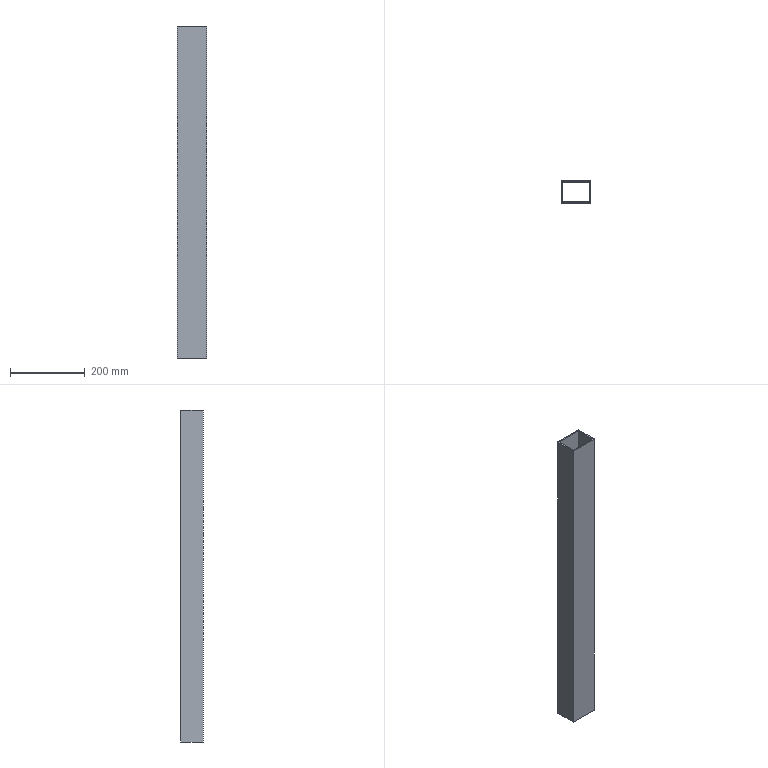Part | STEP file | Guide wheel mechanism revised.sldasm-Part-30 | 1 solid | 12 faces | box 80 x 60 x 890 mm | volume 705411 mm3 | plane 11 | cylinder 1 | commonest cylinder face diameters 500 x1
STEP:
#1=CARTESIAN_POINT('',(-485.,760.,445.));
#2=VERTEX_POINT('',#1);
#3=CARTESIAN_POINT('',(-405.,760.,445.));
#4=VERTEX_POINT('',#3);
#5=CARTESIAN_POINT('',(-405.,760.,445.));
#6=DIRECTION('',(1.,0.,0.));
#7=VECTOR('',#6,1000.);
#8=LINE('',#5,#7);
#9=EDGE_CURVE('',#2,#4,#8,.T.);
#10=ORIENTED_EDGE('',*,*,#9,.F.);
#11=CARTESIAN_POINT('',(-485.,760.,-445.));
#12=VERTEX_POINT('',#11);
#13=CARTESIAN_POINT('',(-485.,760.,545.));
#14=DIRECTION('',(0.,0.,-1.));
#15=VECTOR('',#14,1000.);
#16=LINE('',#13,#15);
#17=EDGE_CURVE('',#2,#12,#16,.T.);
#18=ORIENTED_EDGE('',*,*,#17,.T.);
#19=CARTESIAN_POINT('',(-405.,760.,-445.));
#20=VERTEX_POINT('',#19);
#21=CARTESIAN_POINT('',(-405.,760.,-445.));
#22=DIRECTION('',(1.,0.,0.));
#23=VECTOR('',#22,1000.);
#24=LINE('',#21,#23);
#25=EDGE_CURVE('',#12,#20,#24,.T.);
#26=ORIENTED_EDGE('',*,*,#25,.T.);
#27=CARTESIAN_POINT('',(-405.,760.,545.));
#28=DIRECTION('',(0.,0.,-1.));
#29=VECTOR('',#28,1000.);
#30=LINE('',#27,#29);
#31=EDGE_CURVE('',#4,#20,#30,.T.);
#32=ORIENTED_EDGE('',*,*,#31,.F.);
#33=EDGE_LOOP('',(#10,#18,#26,#32));
#34=FACE_OUTER_BOUND('',#33,.T.);
#35=CARTESIAN_POINT('',(-405.,760.,545.));
#36=DIRECTION('',(0.,1.,0.));
#37=DIRECTION('',(0.,0.,1.));
#38=AXIS2_PLACEMENT_3D('',#35,#36,#37);
#39=PLANE('',#38);
#40=ADVANCED_FACE('',(#34),#39,.F.);
#41=CARTESIAN_POINT('',(-485.,820.,445.));
#42=VERTEX_POINT('',#41);
#43=CARTESIAN_POINT('',(-485.,820.,445.));
#44=DIRECTION('',(0.,-1.,0.));
#45=VECTOR('',#44,1000.);
#46=LINE('',#43,#45);
#47=EDGE_CURVE('',#42,#2,#46,.T.);
#48=ORIENTED_EDGE('',*,*,#47,.F.);
#49=CARTESIAN_POINT('',(-485.,820.,-445.));
#50=VERTEX_POINT('',#49);
#51=CARTESIAN_POINT('',(-485.,820.,545.));
#52=DIRECTION('',(0.,0.,-1.));
#53=VECTOR('',#52,1000.);
#54=LINE('',#51,#53);
#55=EDGE_CURVE('',#42,#50,#54,.T.);
#56=ORIENTED_EDGE('',*,*,#55,.T.);
#57=CARTESIAN_POINT('',(-485.,820.,-445.));
#58=DIRECTION('',(0.,-1.,0.));
#59=VECTOR('',#58,1000.);
#60=LINE('',#57,#59);
#61=EDGE_CURVE('',#50,#12,#60,.T.);
#62=ORIENTED_EDGE('',*,*,#61,.T.);
#63=ORIENTED_EDGE('',*,*,#17,.F.);
#64=EDGE_LOOP('',(#48,#56,#62,#63));
#65=FACE_OUTER_BOUND('',#64,.T.);
#66=CARTESIAN_POINT('',(-485.,820.,545.));
#67=DIRECTION('',(1.,0.,0.));
#68=DIRECTION('',(0.,0.,-1.));
#69=AXIS2_PLACEMENT_3D('',#66,#67,#68);
#70=PLANE('',#69);
#71=ADVANCED_FACE('',(#65),#70,.F.);
#72=CARTESIAN_POINT('',(-405.,820.,445.));
#73=VERTEX_POINT('',#72);
#74=CARTESIAN_POINT('',(-405.,820.,267.168));
#75=VERTEX_POINT('',#74);
#76=CARTESIAN_POINT('',(-405.,820.,545.));
#77=DIRECTION('',(0.,0.,-1.));
#78=VECTOR('',#77,1000.);
#79=LINE('',#76,#78);
#80=EDGE_CURVE('',#73,#75,#79,.T.);
#81=ORIENTED_EDGE('',*,*,#80,.T.);
#82=CARTESIAN_POINT('',(-405.,820.,25.252));
#83=VERTEX_POINT('',#82);
#84=CARTESIAN_POINT('',(-186.21,820.,146.21));
#85=DIRECTION('',(0.,-1.,0.));
#86=DIRECTION('',(0.,0.,-1.));
#87=AXIS2_PLACEMENT_3D('',#84,#85,#86);
#88=CIRCLE('',#87,250.);
#89=EDGE_CURVE('',#75,#83,#88,.T.);
#90=ORIENTED_EDGE('',*,*,#89,.T.);
#91=CARTESIAN_POINT('',(-405.,820.,-445.));
#92=VERTEX_POINT('',#91);
#93=CARTESIAN_POINT('',(-405.,820.,545.));
#94=DIRECTION('',(0.,0.,-1.));
#95=VECTOR('',#94,1000.);
#96=LINE('',#93,#95);
#97=EDGE_CURVE('',#83,#92,#96,.T.);
#98=ORIENTED_EDGE('',*,*,#97,.T.);
#99=CARTESIAN_POINT('',(-405.,820.,-445.));
#100=DIRECTION('',(-1.,0.,0.));
#101=VECTOR('',#100,1000.);
#102=LINE('',#99,#101);
#103=EDGE_CURVE('',#92,#50,#102,.T.);
#104=ORIENTED_EDGE('',*,*,#103,.T.);
#105=ORIENTED_EDGE('',*,*,#55,.F.);
#106=CARTESIAN_POINT('',(-405.,820.,445.));
#107=DIRECTION('',(-1.,0.,0.));
#108=VECTOR('',#107,1000.);
#109=LINE('',#106,#108);
#110=EDGE_CURVE('',#73,#42,#109,.T.);
#111=ORIENTED_EDGE('',*,*,#110,.F.);
#112=EDGE_LOOP('',(#81,#90,#98,#104,#105,#111));
#113=FACE_OUTER_BOUND('',#112,.T.);
#114=CARTESIAN_POINT('',(-405.,820.,545.));
#115=DIRECTION('',(0.,-1.,0.));
#116=DIRECTION('',(0.,0.,-1.));
#117=AXIS2_PLACEMENT_3D('',#114,#115,#116);
#118=PLANE('',#117);
#119=ADVANCED_FACE('',(#113),#118,.F.);
#120=CARTESIAN_POINT('',(-405.,818.01,267.168));
#121=VERTEX_POINT('',#120);
#122=CARTESIAN_POINT('',(-405.,818.01,25.252));
#123=VERTEX_POINT('',#122);
#124=CARTESIAN_POINT('',(-405.,818.01,545.));
#125=DIRECTION('',(0.,0.,-1.));
#126=VECTOR('',#125,1000.);
#127=LINE('',#124,#126);
#128=EDGE_CURVE('',#121,#123,#127,.T.);
#129=ORIENTED_EDGE('',*,*,#128,.F.);
#130=CARTESIAN_POINT('',(-405.,818.01,267.168));
#131=DIRECTION('',(0.,1.,0.));
#132=VECTOR('',#131,1000.);
#133=LINE('',#130,#132);
#134=EDGE_CURVE('',#121,#75,#133,.T.);
#135=ORIENTED_EDGE('',*,*,#134,.T.);
#136=ORIENTED_EDGE('',*,*,#80,.F.);
#137=CARTESIAN_POINT('',(-405.,820.,445.));
#138=DIRECTION('',(0.,1.,0.));
#139=VECTOR('',#138,1000.);
#140=LINE('',#137,#139);
#141=EDGE_CURVE('',#4,#73,#140,.T.);
#142=ORIENTED_EDGE('',*,*,#141,.F.);
#143=ORIENTED_EDGE('',*,*,#31,.T.);
#144=CARTESIAN_POINT('',(-405.,820.,-445.));
#145=DIRECTION('',(0.,1.,0.));
#146=VECTOR('',#145,1000.);
#147=LINE('',#144,#146);
#148=EDGE_CURVE('',#20,#92,#147,.T.);
#149=ORIENTED_EDGE('',*,*,#148,.T.);
#150=ORIENTED_EDGE('',*,*,#97,.F.);
#151=CARTESIAN_POINT('',(-405.,818.01,25.252));
#152=DIRECTION('',(0.,-1.,0.));
#153=VECTOR('',#152,1000.);
#154=LINE('',#151,#153);
#155=EDGE_CURVE('',#83,#123,#154,.T.);
#156=ORIENTED_EDGE('',*,*,#155,.T.);
#157=EDGE_LOOP('',(#129,#135,#136,#142,#143,#149,#150,#156));
#158=FACE_OUTER_BOUND('',#157,.T.);
#159=CARTESIAN_POINT('',(-405.,820.,545.));
#160=DIRECTION('',(-1.,0.,0.));
#161=DIRECTION('',(0.,0.,1.));
#162=AXIS2_PLACEMENT_3D('',#159,#160,#161);
#163=PLANE('',#162);
#164=ADVANCED_FACE('',(#158),#163,.F.);
#165=ORIENTED_EDGE('',*,*,#148,.F.);
#166=ORIENTED_EDGE('',*,*,#25,.F.);
#167=ORIENTED_EDGE('',*,*,#61,.F.);
#168=ORIENTED_EDGE('',*,*,#103,.F.);
#169=EDGE_LOOP('',(#165,#166,#167,#168));
#170=FACE_OUTER_BOUND('',#169,.T.);
#171=CARTESIAN_POINT('',(-482.,763.,-445.));
#172=VERTEX_POINT('',#171);
#173=CARTESIAN_POINT('',(-408.,763.,-445.));
#174=VERTEX_POINT('',#173);
#175=CARTESIAN_POINT('',(-408.,763.,-445.));
#176=DIRECTION('',(1.,0.,0.));
#177=VECTOR('',#176,1000.);
#178=LINE('',#175,#177);
#179=EDGE_CURVE('',#172,#174,#178,.T.);
#180=ORIENTED_EDGE('',*,*,#179,.T.);
#181=CARTESIAN_POINT('',(-408.,817.,-445.));
#182=VERTEX_POINT('',#181);
#183=CARTESIAN_POINT('',(-408.,817.,-445.));
#184=DIRECTION('',(0.,1.,0.));
#185=VECTOR('',#184,1000.);
#186=LINE('',#183,#185);
#187=EDGE_CURVE('',#174,#182,#186,.T.);
#188=ORIENTED_EDGE('',*,*,#187,.T.);
#189=CARTESIAN_POINT('',(-482.,817.,-445.));
#190=VERTEX_POINT('',#189);
#191=CARTESIAN_POINT('',(-408.,817.,-445.));
#192=DIRECTION('',(-1.,0.,0.));
#193=VECTOR('',#192,1000.);
#194=LINE('',#191,#193);
#195=EDGE_CURVE('',#182,#190,#194,.T.);
#196=ORIENTED_EDGE('',*,*,#195,.T.);
#197=CARTESIAN_POINT('',(-482.,817.,-445.));
#198=DIRECTION('',(0.,-1.,0.));
#199=VECTOR('',#198,1000.);
#200=LINE('',#197,#199);
#201=EDGE_CURVE('',#190,#172,#200,.T.);
#202=ORIENTED_EDGE('',*,*,#201,.T.);
#203=EDGE_LOOP('',(#180,#188,#196,#202));
#204=FACE_BOUND('',#203,.T.);
#205=CARTESIAN_POINT('',(0.,0.,-445.));
#206=DIRECTION('',(0.,0.,-1.));
#207=DIRECTION('',(-1.,0.,0.));
#208=AXIS2_PLACEMENT_3D('',#205,#206,#207);
#209=PLANE('',#208);
#210=ADVANCED_FACE('',(#170,#204),#209,.T.);
#211=CARTESIAN_POINT('',(-482.,763.,445.));
#212=VERTEX_POINT('',#211);
#213=CARTESIAN_POINT('',(-482.,763.,545.));
#214=DIRECTION('',(0.,0.,-1.));
#215=VECTOR('',#214,1000.);
#216=LINE('',#213,#215);
#217=EDGE_CURVE('',#212,#172,#216,.T.);
#218=ORIENTED_EDGE('',*,*,#217,.F.);
#219=CARTESIAN_POINT('',(-408.,763.,445.));
#220=VERTEX_POINT('',#219);
#221=CARTESIAN_POINT('',(-408.,763.,445.));
#222=DIRECTION('',(1.,0.,0.));
#223=VECTOR('',#222,1000.);
#224=LINE('',#221,#223);
#225=EDGE_CURVE('',#212,#220,#224,.T.);
#226=ORIENTED_EDGE('',*,*,#225,.T.);
#227=CARTESIAN_POINT('',(-408.,763.,545.));
#228=DIRECTION('',(0.,0.,-1.));
#229=VECTOR('',#228,1000.);
#230=LINE('',#227,#229);
#231=EDGE_CURVE('',#220,#174,#230,.T.);
#232=ORIENTED_EDGE('',*,*,#231,.T.);
#233=ORIENTED_EDGE('',*,*,#179,.F.);
#234=EDGE_LOOP('',(#218,#226,#232,#233));
#235=FACE_OUTER_BOUND('',#234,.T.);
#236=CARTESIAN_POINT('',(-408.,763.,545.));
#237=DIRECTION('',(0.,1.,0.));
#238=DIRECTION('',(0.,0.,1.));
#239=AXIS2_PLACEMENT_3D('',#236,#237,#238);
#240=PLANE('',#239);
#241=ADVANCED_FACE('',(#235),#240,.T.);
#242=CARTESIAN_POINT('',(-482.,817.,445.));
#243=VERTEX_POINT('',#242);
#244=CARTESIAN_POINT('',(-482.,817.,545.));
#245=DIRECTION('',(0.,0.,-1.));
#246=VECTOR('',#245,1000.);
#247=LINE('',#244,#246);
#248=EDGE_CURVE('',#243,#190,#247,.T.);
#249=ORIENTED_EDGE('',*,*,#248,.F.);
#250=CARTESIAN_POINT('',(-482.,817.,445.));
#251=DIRECTION('',(0.,-1.,0.));
#252=VECTOR('',#251,1000.);
#253=LINE('',#250,#252);
#254=EDGE_CURVE('',#243,#212,#253,.T.);
#255=ORIENTED_EDGE('',*,*,#254,.T.);
#256=ORIENTED_EDGE('',*,*,#217,.T.);
#257=ORIENTED_EDGE('',*,*,#201,.F.);
#258=EDGE_LOOP('',(#249,#255,#256,#257));
#259=FACE_OUTER_BOUND('',#258,.T.);
#260=CARTESIAN_POINT('',(-482.,817.,545.));
#261=DIRECTION('',(1.,0.,0.));
#262=DIRECTION('',(0.,0.,-1.));
#263=AXIS2_PLACEMENT_3D('',#260,#261,#262);
#264=PLANE('',#263);
#265=ADVANCED_FACE('',(#259),#264,.T.);
#266=CARTESIAN_POINT('',(-408.,817.,445.));
#267=VERTEX_POINT('',#266);
#268=CARTESIAN_POINT('',(-408.,817.,545.));
#269=DIRECTION('',(0.,0.,-1.));
#270=VECTOR('',#269,1000.);
#271=LINE('',#268,#270);
#272=EDGE_CURVE('',#267,#182,#271,.T.);
#273=ORIENTED_EDGE('',*,*,#272,.F.);
#274=CARTESIAN_POINT('',(-408.,817.,445.));
#275=DIRECTION('',(-1.,0.,0.));
#276=VECTOR('',#275,1000.);
#277=LINE('',#274,#276);
#278=EDGE_CURVE('',#267,#243,#277,.T.);
#279=ORIENTED_EDGE('',*,*,#278,.T.);
#280=ORIENTED_EDGE('',*,*,#248,.T.);
#281=ORIENTED_EDGE('',*,*,#195,.F.);
#282=EDGE_LOOP('',(#273,#279,#280,#281));
#283=FACE_OUTER_BOUND('',#282,.T.);
#284=CARTESIAN_POINT('',(-408.,817.,545.));
#285=DIRECTION('',(0.,-1.,0.));
#286=DIRECTION('',(0.,0.,-1.));
#287=AXIS2_PLACEMENT_3D('',#284,#285,#286);
#288=PLANE('',#287);
#289=ADVANCED_FACE('',(#283),#288,.T.);
#290=ORIENTED_EDGE('',*,*,#231,.F.);
#291=CARTESIAN_POINT('',(-408.,817.,445.));
#292=DIRECTION('',(0.,1.,0.));
#293=VECTOR('',#292,1000.);
#294=LINE('',#291,#293);
#295=EDGE_CURVE('',#220,#267,#294,.T.);
#296=ORIENTED_EDGE('',*,*,#295,.T.);
#297=ORIENTED_EDGE('',*,*,#272,.T.);
#298=ORIENTED_EDGE('',*,*,#187,.F.);
#299=EDGE_LOOP('',(#290,#296,#297,#298));
#300=FACE_OUTER_BOUND('',#299,.T.);
#301=CARTESIAN_POINT('',(-408.,817.,545.));
#302=DIRECTION('',(-1.,0.,0.));
#303=DIRECTION('',(0.,-1.,0.));
#304=AXIS2_PLACEMENT_3D('',#301,#302,#303);
#305=PLANE('',#304);
#306=ADVANCED_FACE('',(#300),#305,.T.);
#307=ORIENTED_EDGE('',*,*,#295,.F.);
#308=ORIENTED_EDGE('',*,*,#225,.F.);
#309=ORIENTED_EDGE('',*,*,#254,.F.);
#310=ORIENTED_EDGE('',*,*,#278,.F.);
#311=EDGE_LOOP('',(#307,#308,#309,#310));
#312=FACE_BOUND('',#311,.T.);
#313=ORIENTED_EDGE('',*,*,#9,.T.);
#314=ORIENTED_EDGE('',*,*,#141,.T.);
#315=ORIENTED_EDGE('',*,*,#110,.T.);
#316=ORIENTED_EDGE('',*,*,#47,.T.);
#317=EDGE_LOOP('',(#313,#314,#315,#316));
#318=FACE_OUTER_BOUND('',#317,.T.);
#319=CARTESIAN_POINT('',(-405.,1970.,445.));
#320=DIRECTION('',(0.,0.,1.));
#321=DIRECTION('',(1.,0.,0.));
#322=AXIS2_PLACEMENT_3D('',#319,#320,#321);
#323=PLANE('',#322);
#324=ADVANCED_FACE('',(#312,#318),#323,.T.);
#325=CARTESIAN_POINT('',(-186.21,818.01,146.21));
#326=DIRECTION('',(0.,1.,0.));
#327=DIRECTION('',(0.,0.,1.));
#328=AXIS2_PLACEMENT_3D('',#325,#326,#327);
#329=CIRCLE('',#328,250.);
#330=EDGE_CURVE('',#123,#121,#329,.T.);
#331=ORIENTED_EDGE('',*,*,#330,.F.);
#332=ORIENTED_EDGE('',*,*,#155,.F.);
#333=ORIENTED_EDGE('',*,*,#89,.F.);
#334=ORIENTED_EDGE('',*,*,#134,.F.);
#335=EDGE_LOOP('',(#331,#332,#333,#334));
#336=FACE_OUTER_BOUND('',#335,.T.);
#337=CARTESIAN_POINT('',(-186.21,818.01,146.21));
#338=DIRECTION('',(0.,1.,0.));
#339=DIRECTION('',(0.,0.,1.));
#340=AXIS2_PLACEMENT_3D('',#337,#338,#339);
#341=CYLINDRICAL_SURFACE('',#340,250.);
#342=ADVANCED_FACE('',(#336),#341,.F.);
#343=ORIENTED_EDGE('',*,*,#128,.T.);
#344=ORIENTED_EDGE('',*,*,#330,.T.);
#345=EDGE_LOOP('',(#343,#344));
#346=FACE_OUTER_BOUND('',#345,.T.);
#347=CARTESIAN_POINT('',(-186.21,818.01,146.21));
#348=DIRECTION('',(0.,1.,0.));
#349=DIRECTION('',(0.,0.,1.));
#350=AXIS2_PLACEMENT_3D('',#347,#348,#349);
#351=PLANE('',#350);
#352=ADVANCED_FACE('',(#346),#351,.T.);
#353=CLOSED_SHELL('',(#40,#71,#119,#164,#210,#241,#265,#289,#306,#324,#342,#352));
#354=MANIFOLD_SOLID_BREP('',#353);
#355=CARTESIAN_POINT('',(0.,0.,0.));
#356=DIRECTION('',(0.,0.,1.));
#357=DIRECTION('',(1.,0.,0.));
#358=AXIS2_PLACEMENT_3D('',#355,#356,#357);
#359=(LENGTH_UNIT()NAMED_UNIT(*)SI_UNIT(.MILLI.,.METRE.));
#360=UNCERTAINTY_MEASURE_WITH_UNIT(LENGTH_MEASURE(0.00001),#359,'','');
#361=(NAMED_UNIT(*)PLANE_ANGLE_UNIT()SI_UNIT($,.RADIAN.));
#362=(NAMED_UNIT(*)SI_UNIT($,.STERADIAN.)SOLID_ANGLE_UNIT());
#363=(GEOMETRIC_REPRESENTATION_CONTEXT(3)GLOBAL_UNCERTAINTY_ASSIGNED_CONTEXT((#360))GLOBAL_UNIT_ASSIGNED_CONTEXT((#359,#361,#362))REPRESENTATION_CONTEXT('',''));
#364=ADVANCED_BREP_SHAPE_REPRESENTATION('',(#354,#358),#363);